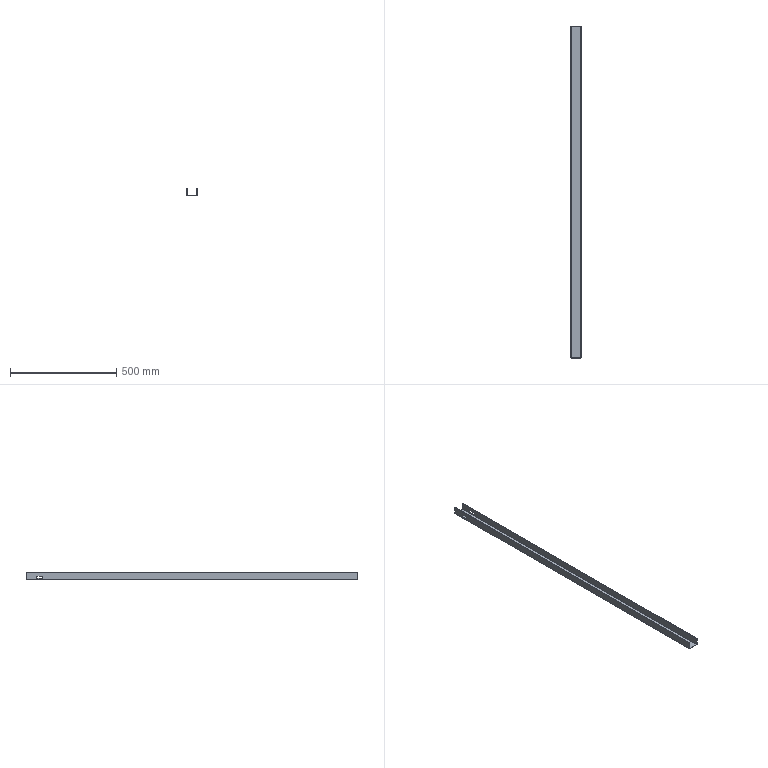Part | SolidWorks | features SplitBody 1 | 1 solid | 30 faces | box 50 x 1562 x 35 mm | volume 271759 mm3 | plane 26 | cylinder 4 | commonest cylinder face diameters 0.2 x2 3.2 x2
STEP:
#1=CARTESIAN_POINT('',(-25.,0.,-298.4));
#2=VERTEX_POINT('',#1);
#3=CARTESIAN_POINT('',(-23.5,0.,-298.4));
#4=VERTEX_POINT('',#3);
#5=CARTESIAN_POINT('',(-25.,0.,-298.4));
#6=DIRECTION('',(1.,0.,0.));
#7=VECTOR('',#6,1000.);
#8=LINE('',#5,#7);
#9=EDGE_CURVE('',#2,#4,#8,.T.);
#10=ORIENTED_EDGE('',*,*,#9,.F.);
#11=CARTESIAN_POINT('',(-23.4,0.,-300.));
#12=VERTEX_POINT('',#11);
#13=CARTESIAN_POINT('',(-23.4,0.,-298.4));
#14=DIRECTION('',(0.,-1.,0.));
#15=DIRECTION('',(0.,0.,1.));
#16=AXIS2_PLACEMENT_3D('',#13,#14,#15);
#17=CIRCLE('',#16,1.6);
#18=EDGE_CURVE('',#2,#12,#17,.T.);
#19=ORIENTED_EDGE('',*,*,#18,.T.);
#20=CARTESIAN_POINT('',(-23.4,0.,-298.5));
#21=VERTEX_POINT('',#20);
#22=CARTESIAN_POINT('',(-23.4,0.,-298.5));
#23=DIRECTION('',(0.,0.,-1.));
#24=VECTOR('',#23,1000.);
#25=LINE('',#22,#24);
#26=EDGE_CURVE('',#21,#12,#25,.T.);
#27=ORIENTED_EDGE('',*,*,#26,.F.);
#28=CARTESIAN_POINT('',(-23.4,0.,-298.4));
#29=DIRECTION('',(0.,-1.,0.));
#30=DIRECTION('',(1.,0.,0.));
#31=AXIS2_PLACEMENT_3D('',#28,#29,#30);
#32=CIRCLE('',#31,0.1);
#33=EDGE_CURVE('',#4,#21,#32,.T.);
#34=ORIENTED_EDGE('',*,*,#33,.F.);
#35=EDGE_LOOP('',(#10,#19,#27,#34));
#36=FACE_OUTER_BOUND('',#35,.T.);
#37=CARTESIAN_POINT('',(-25.,0.,-298.4));
#38=DIRECTION('',(0.,-1.,0.));
#39=DIRECTION('',(0.,0.,-1.));
#40=AXIS2_PLACEMENT_3D('',#37,#38,#39);
#41=PLANE('',#40);
#42=ADVANCED_FACE('',(#36),#41,.T.);
#43=CARTESIAN_POINT('',(-25.,0.,-265.));
#44=VERTEX_POINT('',#43);
#45=CARTESIAN_POINT('',(-25.,0.,-265.));
#46=DIRECTION('',(0.,0.,-1.));
#47=VECTOR('',#46,1000.);
#48=LINE('',#45,#47);
#49=EDGE_CURVE('',#44,#2,#48,.T.);
#50=ORIENTED_EDGE('',*,*,#49,.T.);
#51=ORIENTED_EDGE('',*,*,#9,.T.);
#52=CARTESIAN_POINT('',(-23.5,0.,-265.));
#53=VERTEX_POINT('',#52);
#54=CARTESIAN_POINT('',(-23.5,0.,-265.));
#55=DIRECTION('',(0.,0.,-1.));
#56=VECTOR('',#55,1000.);
#57=LINE('',#54,#56);
#58=EDGE_CURVE('',#53,#4,#57,.T.);
#59=ORIENTED_EDGE('',*,*,#58,.F.);
#60=CARTESIAN_POINT('',(-23.5,0.,-265.));
#61=DIRECTION('',(-1.,0.,0.));
#62=VECTOR('',#61,1000.);
#63=LINE('',#60,#62);
#64=EDGE_CURVE('',#53,#44,#63,.T.);
#65=ORIENTED_EDGE('',*,*,#64,.T.);
#66=EDGE_LOOP('',(#50,#51,#59,#65));
#67=FACE_OUTER_BOUND('',#66,.T.);
#68=CARTESIAN_POINT('',(-23.4,0.,-298.5));
#69=DIRECTION('',(0.,-1.,0.));
#70=DIRECTION('',(0.,0.,-1.));
#71=AXIS2_PLACEMENT_3D('',#68,#69,#70);
#72=PLANE('',#71);
#73=ADVANCED_FACE('',(#67),#72,.T.);
#74=CARTESIAN_POINT('',(23.4,0.,-300.));
#75=VERTEX_POINT('',#74);
#76=CARTESIAN_POINT('',(23.4,0.,-298.5));
#77=VERTEX_POINT('',#76);
#78=CARTESIAN_POINT('',(23.4,0.,-300.));
#79=DIRECTION('',(0.,0.,1.));
#80=VECTOR('',#79,1000.);
#81=LINE('',#78,#80);
#82=EDGE_CURVE('',#75,#77,#81,.T.);
#83=ORIENTED_EDGE('',*,*,#82,.F.);
#84=CARTESIAN_POINT('',(25.,0.,-298.4));
#85=VERTEX_POINT('',#84);
#86=CARTESIAN_POINT('',(23.4,0.,-298.4));
#87=DIRECTION('',(0.,-1.,0.));
#88=DIRECTION('',(0.,0.,1.));
#89=AXIS2_PLACEMENT_3D('',#86,#87,#88);
#90=CIRCLE('',#89,1.6);
#91=EDGE_CURVE('',#75,#85,#90,.T.);
#92=ORIENTED_EDGE('',*,*,#91,.T.);
#93=CARTESIAN_POINT('',(23.5,0.,-298.4));
#94=VERTEX_POINT('',#93);
#95=CARTESIAN_POINT('',(23.5,0.,-298.4));
#96=DIRECTION('',(1.,0.,0.));
#97=VECTOR('',#96,1000.);
#98=LINE('',#95,#97);
#99=EDGE_CURVE('',#94,#85,#98,.T.);
#100=ORIENTED_EDGE('',*,*,#99,.F.);
#101=CARTESIAN_POINT('',(23.4,0.,-298.4));
#102=DIRECTION('',(0.,-1.,0.));
#103=DIRECTION('',(1.,0.,0.));
#104=AXIS2_PLACEMENT_3D('',#101,#102,#103);
#105=CIRCLE('',#104,0.1);
#106=EDGE_CURVE('',#77,#94,#105,.T.);
#107=ORIENTED_EDGE('',*,*,#106,.F.);
#108=EDGE_LOOP('',(#83,#92,#100,#107));
#109=FACE_OUTER_BOUND('',#108,.T.);
#110=CARTESIAN_POINT('',(23.4,0.,-300.));
#111=DIRECTION('',(0.,-1.,0.));
#112=DIRECTION('',(0.,0.,-1.));
#113=AXIS2_PLACEMENT_3D('',#110,#111,#112);
#114=PLANE('',#113);
#115=ADVANCED_FACE('',(#109),#114,.T.);
#116=CARTESIAN_POINT('',(-25.,0.,-300.));
#117=DIRECTION('',(1.,0.,0.));
#118=VECTOR('',#117,1000.);
#119=LINE('',#116,#118);
#120=EDGE_CURVE('',#12,#75,#119,.T.);
#121=ORIENTED_EDGE('',*,*,#120,.T.);
#122=ORIENTED_EDGE('',*,*,#82,.T.);
#123=CARTESIAN_POINT('',(-25.,0.,-298.5));
#124=DIRECTION('',(1.,0.,0.));
#125=VECTOR('',#124,1000.);
#126=LINE('',#123,#125);
#127=EDGE_CURVE('',#21,#77,#126,.T.);
#128=ORIENTED_EDGE('',*,*,#127,.F.);
#129=ORIENTED_EDGE('',*,*,#26,.T.);
#130=EDGE_LOOP('',(#121,#122,#128,#129));
#131=FACE_OUTER_BOUND('',#130,.T.);
#132=CARTESIAN_POINT('',(23.5,0.,-298.4));
#133=DIRECTION('',(0.,-1.,0.));
#134=DIRECTION('',(0.,0.,-1.));
#135=AXIS2_PLACEMENT_3D('',#132,#133,#134);
#136=PLANE('',#135);
#137=ADVANCED_FACE('',(#131),#136,.T.);
#138=CARTESIAN_POINT('',(23.5,1486.25,-283.));
#139=VERTEX_POINT('',#138);
#140=CARTESIAN_POINT('',(23.5,1486.25,-293.));
#141=VERTEX_POINT('',#140);
#142=CARTESIAN_POINT('',(23.5,1486.25,-300.));
#143=DIRECTION('',(0.,0.,-1.));
#144=VECTOR('',#143,1000.);
#145=LINE('',#142,#144);
#146=EDGE_CURVE('',#139,#141,#145,.T.);
#147=ORIENTED_EDGE('',*,*,#146,.T.);
#148=CARTESIAN_POINT('',(23.5,1511.25,-293.));
#149=VERTEX_POINT('',#148);
#150=CARTESIAN_POINT('',(23.5,1623.533,-293.));
#151=DIRECTION('',(0.,1.,0.));
#152=VECTOR('',#151,1000.);
#153=LINE('',#150,#152);
#154=EDGE_CURVE('',#141,#149,#153,.T.);
#155=ORIENTED_EDGE('',*,*,#154,.T.);
#156=CARTESIAN_POINT('',(23.5,1511.25,-283.));
#157=VERTEX_POINT('',#156);
#158=CARTESIAN_POINT('',(23.5,1511.25,-300.));
#159=DIRECTION('',(0.,0.,1.));
#160=VECTOR('',#159,1000.);
#161=LINE('',#158,#160);
#162=EDGE_CURVE('',#149,#157,#161,.T.);
#163=ORIENTED_EDGE('',*,*,#162,.T.);
#164=CARTESIAN_POINT('',(23.5,1623.533,-283.));
#165=DIRECTION('',(0.,-1.,0.));
#166=VECTOR('',#165,1000.);
#167=LINE('',#164,#166);
#168=EDGE_CURVE('',#157,#139,#167,.T.);
#169=ORIENTED_EDGE('',*,*,#168,.T.);
#170=EDGE_LOOP('',(#147,#155,#163,#169));
#171=FACE_BOUND('',#170,.T.);
#172=CARTESIAN_POINT('',(23.5,1562.5,-298.4));
#173=VERTEX_POINT('',#172);
#174=CARTESIAN_POINT('',(23.5,1562.5,-265.));
#175=VERTEX_POINT('',#174);
#176=CARTESIAN_POINT('',(23.5,1562.5,-300.));
#177=DIRECTION('',(0.,0.,1.));
#178=VECTOR('',#177,1000.);
#179=LINE('',#176,#178);
#180=EDGE_CURVE('',#173,#175,#179,.T.);
#181=ORIENTED_EDGE('',*,*,#180,.F.);
#182=CARTESIAN_POINT('',(23.5,1623.533,-298.4));
#183=DIRECTION('',(0.,-1.,0.));
#184=VECTOR('',#183,1000.);
#185=LINE('',#182,#184);
#186=EDGE_CURVE('',#173,#94,#185,.T.);
#187=ORIENTED_EDGE('',*,*,#186,.T.);
#188=CARTESIAN_POINT('',(23.5,0.,-265.));
#189=VERTEX_POINT('',#188);
#190=CARTESIAN_POINT('',(23.5,0.,-300.));
#191=DIRECTION('',(0.,0.,1.));
#192=VECTOR('',#191,1000.);
#193=LINE('',#190,#192);
#194=EDGE_CURVE('',#94,#189,#193,.T.);
#195=ORIENTED_EDGE('',*,*,#194,.T.);
#196=CARTESIAN_POINT('',(23.5,1623.533,-265.));
#197=DIRECTION('',(0.,-1.,0.));
#198=VECTOR('',#197,1000.);
#199=LINE('',#196,#198);
#200=EDGE_CURVE('',#175,#189,#199,.T.);
#201=ORIENTED_EDGE('',*,*,#200,.F.);
#202=EDGE_LOOP('',(#181,#187,#195,#201));
#203=FACE_OUTER_BOUND('',#202,.T.);
#204=CARTESIAN_POINT('',(23.5,1623.533,-300.));
#205=DIRECTION('',(1.,0.,0.));
#206=DIRECTION('',(0.,0.,-1.));
#207=AXIS2_PLACEMENT_3D('',#204,#205,#206);
#208=PLANE('',#207);
#209=ADVANCED_FACE('',(#171,#203),#208,.F.);
#210=CARTESIAN_POINT('',(25.,1562.5,-265.));
#211=VERTEX_POINT('',#210);
#212=CARTESIAN_POINT('',(25.,0.,-265.));
#213=VERTEX_POINT('',#212);
#214=CARTESIAN_POINT('',(25.,1623.533,-265.));
#215=DIRECTION('',(0.,-1.,0.));
#216=VECTOR('',#215,1000.);
#217=LINE('',#214,#216);
#218=EDGE_CURVE('',#211,#213,#217,.T.);
#219=ORIENTED_EDGE('',*,*,#218,.F.);
#220=CARTESIAN_POINT('',(25.,1562.5,-265.));
#221=DIRECTION('',(-1.,0.,0.));
#222=VECTOR('',#221,1000.);
#223=LINE('',#220,#222);
#224=EDGE_CURVE('',#211,#175,#223,.T.);
#225=ORIENTED_EDGE('',*,*,#224,.T.);
#226=ORIENTED_EDGE('',*,*,#200,.T.);
#227=CARTESIAN_POINT('',(25.,0.,-265.));
#228=DIRECTION('',(-1.,0.,0.));
#229=VECTOR('',#228,1000.);
#230=LINE('',#227,#229);
#231=EDGE_CURVE('',#213,#189,#230,.T.);
#232=ORIENTED_EDGE('',*,*,#231,.F.);
#233=EDGE_LOOP('',(#219,#225,#226,#232));
#234=FACE_OUTER_BOUND('',#233,.T.);
#235=CARTESIAN_POINT('',(25.,1623.533,-265.));
#236=DIRECTION('',(0.,0.,1.));
#237=DIRECTION('',(1.,0.,0.));
#238=AXIS2_PLACEMENT_3D('',#235,#236,#237);
#239=PLANE('',#238);
#240=ADVANCED_FACE('',(#234),#239,.T.);
#241=CARTESIAN_POINT('',(25.,1486.25,-293.));
#242=VERTEX_POINT('',#241);
#243=CARTESIAN_POINT('',(25.,1511.25,-293.));
#244=VERTEX_POINT('',#243);
#245=CARTESIAN_POINT('',(25.,1511.25,-293.));
#246=DIRECTION('',(0.,1.,0.));
#247=VECTOR('',#246,1000.);
#248=LINE('',#245,#247);
#249=EDGE_CURVE('',#242,#244,#248,.T.);
#250=ORIENTED_EDGE('',*,*,#249,.F.);
#251=CARTESIAN_POINT('',(25.,1486.25,-283.));
#252=VERTEX_POINT('',#251);
#253=CARTESIAN_POINT('',(25.,1486.25,-293.));
#254=DIRECTION('',(0.,0.,-1.));
#255=VECTOR('',#254,1000.);
#256=LINE('',#253,#255);
#257=EDGE_CURVE('',#252,#242,#256,.T.);
#258=ORIENTED_EDGE('',*,*,#257,.F.);
#259=CARTESIAN_POINT('',(25.,1511.25,-283.));
#260=VERTEX_POINT('',#259);
#261=CARTESIAN_POINT('',(25.,1511.25,-283.));
#262=DIRECTION('',(0.,-1.,0.));
#263=VECTOR('',#262,1000.);
#264=LINE('',#261,#263);
#265=EDGE_CURVE('',#260,#252,#264,.T.);
#266=ORIENTED_EDGE('',*,*,#265,.F.);
#267=CARTESIAN_POINT('',(25.,1511.25,-293.));
#268=DIRECTION('',(0.,0.,1.));
#269=VECTOR('',#268,1000.);
#270=LINE('',#267,#269);
#271=EDGE_CURVE('',#244,#260,#270,.T.);
#272=ORIENTED_EDGE('',*,*,#271,.F.);
#273=EDGE_LOOP('',(#250,#258,#266,#272));
#274=FACE_BOUND('',#273,.T.);
#275=CARTESIAN_POINT('',(25.,1562.5,-298.4));
#276=VERTEX_POINT('',#275);
#277=CARTESIAN_POINT('',(25.,1623.533,-298.4));
#278=DIRECTION('',(0.,-1.,0.));
#279=VECTOR('',#278,1000.);
#280=LINE('',#277,#279);
#281=EDGE_CURVE('',#276,#85,#280,.T.);
#282=ORIENTED_EDGE('',*,*,#281,.F.);
#283=CARTESIAN_POINT('',(25.,1562.5,-300.));
#284=DIRECTION('',(0.,0.,1.));
#285=VECTOR('',#284,1000.);
#286=LINE('',#283,#285);
#287=EDGE_CURVE('',#276,#211,#286,.T.);
#288=ORIENTED_EDGE('',*,*,#287,.T.);
#289=ORIENTED_EDGE('',*,*,#218,.T.);
#290=CARTESIAN_POINT('',(25.,0.,-300.));
#291=DIRECTION('',(0.,0.,1.));
#292=VECTOR('',#291,1000.);
#293=LINE('',#290,#292);
#294=EDGE_CURVE('',#85,#213,#293,.T.);
#295=ORIENTED_EDGE('',*,*,#294,.F.);
#296=EDGE_LOOP('',(#282,#288,#289,#295));
#297=FACE_OUTER_BOUND('',#296,.T.);
#298=CARTESIAN_POINT('',(25.,1623.533,-300.));
#299=DIRECTION('',(1.,0.,0.));
#300=DIRECTION('',(0.,0.,-1.));
#301=AXIS2_PLACEMENT_3D('',#298,#299,#300);
#302=PLANE('',#301);
#303=ADVANCED_FACE('',(#274,#297),#302,.T.);
#304=CARTESIAN_POINT('',(23.4,1562.5,-300.));
#305=VERTEX_POINT('',#304);
#306=CARTESIAN_POINT('',(23.4,1623.533,-300.));
#307=DIRECTION('',(0.,-1.,0.));
#308=VECTOR('',#307,1000.);
#309=LINE('',#306,#308);
#310=EDGE_CURVE('',#305,#75,#309,.T.);
#311=ORIENTED_EDGE('',*,*,#310,.F.);
#312=CARTESIAN_POINT('',(23.4,1562.5,-298.4));
#313=DIRECTION('',(0.,1.,0.));
#314=DIRECTION('',(0.,0.,-1.));
#315=AXIS2_PLACEMENT_3D('',#312,#313,#314);
#316=CIRCLE('',#315,1.6);
#317=EDGE_CURVE('',#276,#305,#316,.T.);
#318=ORIENTED_EDGE('',*,*,#317,.F.);
#319=ORIENTED_EDGE('',*,*,#281,.T.);
#320=ORIENTED_EDGE('',*,*,#91,.F.);
#321=EDGE_LOOP('',(#311,#318,#319,#320));
#322=FACE_OUTER_BOUND('',#321,.T.);
#323=CARTESIAN_POINT('',(23.4,1623.533,-298.4));
#324=DIRECTION('',(0.,-1.,0.));
#325=DIRECTION('',(0.,0.,-1.));
#326=AXIS2_PLACEMENT_3D('',#323,#324,#325);
#327=CYLINDRICAL_SURFACE('',#326,1.6);
#328=ADVANCED_FACE('',(#322),#327,.T.);
#329=CARTESIAN_POINT('',(-23.4,1562.5,-300.));
#330=VERTEX_POINT('',#329);
#331=CARTESIAN_POINT('',(-23.4,1623.533,-300.));
#332=DIRECTION('',(0.,-1.,0.));
#333=VECTOR('',#332,1000.);
#334=LINE('',#331,#333);
#335=EDGE_CURVE('',#330,#12,#334,.T.);
#336=ORIENTED_EDGE('',*,*,#335,.F.);
#337=CARTESIAN_POINT('',(-25.,1562.5,-300.));
#338=DIRECTION('',(1.,0.,0.));
#339=VECTOR('',#338,1000.);
#340=LINE('',#337,#339);
#341=EDGE_CURVE('',#330,#305,#340,.T.);
#342=ORIENTED_EDGE('',*,*,#341,.T.);
#343=ORIENTED_EDGE('',*,*,#310,.T.);
#344=ORIENTED_EDGE('',*,*,#120,.F.);
#345=EDGE_LOOP('',(#336,#342,#343,#344));
#346=FACE_OUTER_BOUND('',#345,.T.);
#347=CARTESIAN_POINT('',(-25.,1623.533,-300.));
#348=DIRECTION('',(0.,0.,-1.));
#349=DIRECTION('',(-1.,0.,0.));
#350=AXIS2_PLACEMENT_3D('',#347,#348,#349);
#351=PLANE('',#350);
#352=ADVANCED_FACE('',(#346),#351,.T.);
#353=CARTESIAN_POINT('',(-25.,1562.5,-298.4));
#354=VERTEX_POINT('',#353);
#355=CARTESIAN_POINT('',(-25.,1623.533,-298.4));
#356=DIRECTION('',(0.,-1.,0.));
#357=VECTOR('',#356,1000.);
#358=LINE('',#355,#357);
#359=EDGE_CURVE('',#354,#2,#358,.T.);
#360=ORIENTED_EDGE('',*,*,#359,.F.);
#361=CARTESIAN_POINT('',(-23.4,1562.5,-298.4));
#362=DIRECTION('',(0.,1.,0.));
#363=DIRECTION('',(0.,0.,-1.));
#364=AXIS2_PLACEMENT_3D('',#361,#362,#363);
#365=CIRCLE('',#364,1.6);
#366=EDGE_CURVE('',#330,#354,#365,.T.);
#367=ORIENTED_EDGE('',*,*,#366,.F.);
#368=ORIENTED_EDGE('',*,*,#335,.T.);
#369=ORIENTED_EDGE('',*,*,#18,.F.);
#370=EDGE_LOOP('',(#360,#367,#368,#369));
#371=FACE_OUTER_BOUND('',#370,.T.);
#372=CARTESIAN_POINT('',(-23.4,1623.533,-298.4));
#373=DIRECTION('',(0.,-1.,0.));
#374=DIRECTION('',(0.,0.,-1.));
#375=AXIS2_PLACEMENT_3D('',#372,#373,#374);
#376=CYLINDRICAL_SURFACE('',#375,1.6);
#377=ADVANCED_FACE('',(#371),#376,.T.);
#378=CARTESIAN_POINT('',(-25.,1511.25,-293.));
#379=VERTEX_POINT('',#378);
#380=CARTESIAN_POINT('',(-25.,1486.25,-293.));
#381=VERTEX_POINT('',#380);
#382=CARTESIAN_POINT('',(-25.,1623.533,-293.));
#383=DIRECTION('',(0.,-1.,0.));
#384=VECTOR('',#383,1000.);
#385=LINE('',#382,#384);
#386=EDGE_CURVE('',#379,#381,#385,.T.);
#387=ORIENTED_EDGE('',*,*,#386,.F.);
#388=CARTESIAN_POINT('',(-25.,1511.25,-283.));
#389=VERTEX_POINT('',#388);
#390=CARTESIAN_POINT('',(-25.,1511.25,-265.));
#391=DIRECTION('',(0.,0.,-1.));
#392=VECTOR('',#391,1000.);
#393=LINE('',#390,#392);
#394=EDGE_CURVE('',#389,#379,#393,.T.);
#395=ORIENTED_EDGE('',*,*,#394,.F.);
#396=CARTESIAN_POINT('',(-25.,1486.25,-283.));
#397=VERTEX_POINT('',#396);
#398=CARTESIAN_POINT('',(-25.,1623.533,-283.));
#399=DIRECTION('',(0.,1.,0.));
#400=VECTOR('',#399,1000.);
#401=LINE('',#398,#400);
#402=EDGE_CURVE('',#397,#389,#401,.T.);
#403=ORIENTED_EDGE('',*,*,#402,.F.);
#404=CARTESIAN_POINT('',(-25.,1486.25,-265.));
#405=DIRECTION('',(0.,0.,1.));
#406=VECTOR('',#405,1000.);
#407=LINE('',#404,#406);
#408=EDGE_CURVE('',#381,#397,#407,.T.);
#409=ORIENTED_EDGE('',*,*,#408,.F.);
#410=EDGE_LOOP('',(#387,#395,#403,#409));
#411=FACE_BOUND('',#410,.T.);
#412=CARTESIAN_POINT('',(-25.,1562.5,-265.));
#413=VERTEX_POINT('',#412);
#414=CARTESIAN_POINT('',(-25.,1623.533,-265.));
#415=DIRECTION('',(0.,-1.,0.));
#416=VECTOR('',#415,1000.);
#417=LINE('',#414,#416);
#418=EDGE_CURVE('',#413,#44,#417,.T.);
#419=ORIENTED_EDGE('',*,*,#418,.F.);
#420=CARTESIAN_POINT('',(-25.,1562.5,-265.));
#421=DIRECTION('',(0.,0.,-1.));
#422=VECTOR('',#421,1000.);
#423=LINE('',#420,#422);
#424=EDGE_CURVE('',#413,#354,#423,.T.);
#425=ORIENTED_EDGE('',*,*,#424,.T.);
#426=ORIENTED_EDGE('',*,*,#359,.T.);
#427=ORIENTED_EDGE('',*,*,#49,.F.);
#428=EDGE_LOOP('',(#419,#425,#426,#427));
#429=FACE_OUTER_BOUND('',#428,.T.);
#430=CARTESIAN_POINT('',(-25.,1623.533,-265.));
#431=DIRECTION('',(-1.,0.,0.));
#432=DIRECTION('',(0.,0.,1.));
#433=AXIS2_PLACEMENT_3D('',#430,#431,#432);
#434=PLANE('',#433);
#435=ADVANCED_FACE('',(#411,#429),#434,.T.);
#436=CARTESIAN_POINT('',(-23.5,1562.5,-265.));
#437=VERTEX_POINT('',#436);
#438=CARTESIAN_POINT('',(-23.5,1623.533,-265.));
#439=DIRECTION('',(0.,-1.,0.));
#440=VECTOR('',#439,1000.);
#441=LINE('',#438,#440);
#442=EDGE_CURVE('',#437,#53,#441,.T.);
#443=ORIENTED_EDGE('',*,*,#442,.F.);
#444=CARTESIAN_POINT('',(-23.5,1562.5,-265.));
#445=DIRECTION('',(-1.,0.,0.));
#446=VECTOR('',#445,1000.);
#447=LINE('',#444,#446);
#448=EDGE_CURVE('',#437,#413,#447,.T.);
#449=ORIENTED_EDGE('',*,*,#448,.T.);
#450=ORIENTED_EDGE('',*,*,#418,.T.);
#451=ORIENTED_EDGE('',*,*,#64,.F.);
#452=EDGE_LOOP('',(#443,#449,#450,#451));
#453=FACE_OUTER_BOUND('',#452,.T.);
#454=CARTESIAN_POINT('',(-23.5,1623.533,-265.));
#455=DIRECTION('',(0.,0.,1.));
#456=DIRECTION('',(1.,0.,0.));
#457=AXIS2_PLACEMENT_3D('',#454,#455,#456);
#458=PLANE('',#457);
#459=ADVANCED_FACE('',(#453),#458,.T.);
#460=CARTESIAN_POINT('',(-23.5,1511.25,-283.));
#461=VERTEX_POINT('',#460);
#462=CARTESIAN_POINT('',(-23.5,1511.25,-293.));
#463=VERTEX_POINT('',#462);
#464=CARTESIAN_POINT('',(-23.5,1511.25,-265.));
#465=DIRECTION('',(0.,0.,-1.));
#466=VECTOR('',#465,1000.);
#467=LINE('',#464,#466);
#468=EDGE_CURVE('',#461,#463,#467,.T.);
#469=ORIENTED_EDGE('',*,*,#468,.T.);
#470=CARTESIAN_POINT('',(-23.5,1486.25,-293.));
#471=VERTEX_POINT('',#470);
#472=CARTESIAN_POINT('',(-23.5,1623.533,-293.));
#473=DIRECTION('',(0.,-1.,0.));
#474=VECTOR('',#473,1000.);
#475=LINE('',#472,#474);
#476=EDGE_CURVE('',#463,#471,#475,.T.);
#477=ORIENTED_EDGE('',*,*,#476,.T.);
#478=CARTESIAN_POINT('',(-23.5,1486.25,-283.));
#479=VERTEX_POINT('',#478);
#480=CARTESIAN_POINT('',(-23.5,1486.25,-265.));
#481=DIRECTION('',(0.,0.,1.));
#482=VECTOR('',#481,1000.);
#483=LINE('',#480,#482);
#484=EDGE_CURVE('',#471,#479,#483,.T.);
#485=ORIENTED_EDGE('',*,*,#484,.T.);
#486=CARTESIAN_POINT('',(-23.5,1623.533,-283.));
#487=DIRECTION('',(0.,1.,0.));
#488=VECTOR('',#487,1000.);
#489=LINE('',#486,#488);
#490=EDGE_CURVE('',#479,#461,#489,.T.);
#491=ORIENTED_EDGE('',*,*,#490,.T.);
#492=EDGE_LOOP('',(#469,#477,#485,#491));
#493=FACE_BOUND('',#492,.T.);
#494=CARTESIAN_POINT('',(-23.5,1562.5,-298.4));
#495=VERTEX_POINT('',#494);
#496=CARTESIAN_POINT('',(-23.5,1562.5,-265.));
#497=DIRECTION('',(0.,0.,-1.));
#498=VECTOR('',#497,1000.);
#499=LINE('',#496,#498);
#500=EDGE_CURVE('',#437,#495,#499,.T.);
#501=ORIENTED_EDGE('',*,*,#500,.F.);
#502=ORIENTED_EDGE('',*,*,#442,.T.);
#503=ORIENTED_EDGE('',*,*,#58,.T.);
#504=CARTESIAN_POINT('',(-23.5,1623.533,-298.4));
#505=DIRECTION('',(0.,-1.,0.));
#506=VECTOR('',#505,1000.);
#507=LINE('',#504,#506);
#508=EDGE_CURVE('',#495,#4,#507,.T.);
#509=ORIENTED_EDGE('',*,*,#508,.F.);
#510=EDGE_LOOP('',(#501,#502,#503,#509));
#511=FACE_OUTER_BOUND('',#510,.T.);
#512=CARTESIAN_POINT('',(-23.5,1623.533,-265.));
#513=DIRECTION('',(-1.,0.,0.));
#514=DIRECTION('',(0.,0.,1.));
#515=AXIS2_PLACEMENT_3D('',#512,#513,#514);
#516=PLANE('',#515);
#517=ADVANCED_FACE('',(#493,#511),#516,.F.);
#518=CARTESIAN_POINT('',(-23.4,1562.5,-298.5));
#519=VERTEX_POINT('',#518);
#520=CARTESIAN_POINT('',(-23.4,1562.5,-298.4));
#521=DIRECTION('',(0.,-1.,0.));
#522=DIRECTION('',(0.,0.,1.));
#523=AXIS2_PLACEMENT_3D('',#520,#521,#522);
#524=CIRCLE('',#523,0.1);
#525=EDGE_CURVE('',#495,#519,#524,.T.);
#526=ORIENTED_EDGE('',*,*,#525,.F.);
#527=ORIENTED_EDGE('',*,*,#508,.T.);
#528=ORIENTED_EDGE('',*,*,#33,.T.);
#529=CARTESIAN_POINT('',(-23.4,1623.533,-298.5));
#530=DIRECTION('',(0.,-1.,0.));
#531=VECTOR('',#530,1000.);
#532=LINE('',#529,#531);
#533=EDGE_CURVE('',#519,#21,#532,.T.);
#534=ORIENTED_EDGE('',*,*,#533,.F.);
#535=EDGE_LOOP('',(#526,#527,#528,#534));
#536=FACE_OUTER_BOUND('',#535,.T.);
#537=CARTESIAN_POINT('',(-23.4,1623.533,-298.4));
#538=DIRECTION('',(0.,-1.,0.));
#539=DIRECTION('',(0.,0.,-1.));
#540=AXIS2_PLACEMENT_3D('',#537,#538,#539);
#541=CYLINDRICAL_SURFACE('',#540,0.1);
#542=ADVANCED_FACE('',(#536),#541,.F.);
#543=CARTESIAN_POINT('',(23.4,1562.5,-298.5));
#544=VERTEX_POINT('',#543);
#545=CARTESIAN_POINT('',(-25.,1562.5,-298.5));
#546=DIRECTION('',(1.,0.,0.));
#547=VECTOR('',#546,1000.);
#548=LINE('',#545,#547);
#549=EDGE_CURVE('',#519,#544,#548,.T.);
#550=ORIENTED_EDGE('',*,*,#549,.F.);
#551=ORIENTED_EDGE('',*,*,#533,.T.);
#552=ORIENTED_EDGE('',*,*,#127,.T.);
#553=CARTESIAN_POINT('',(23.4,1623.533,-298.5));
#554=DIRECTION('',(0.,-1.,0.));
#555=VECTOR('',#554,1000.);
#556=LINE('',#553,#555);
#557=EDGE_CURVE('',#544,#77,#556,.T.);
#558=ORIENTED_EDGE('',*,*,#557,.F.);
#559=EDGE_LOOP('',(#550,#551,#552,#558));
#560=FACE_OUTER_BOUND('',#559,.T.);
#561=CARTESIAN_POINT('',(-25.,1623.533,-298.5));
#562=DIRECTION('',(0.,0.,-1.));
#563=DIRECTION('',(-1.,0.,0.));
#564=AXIS2_PLACEMENT_3D('',#561,#562,#563);
#565=PLANE('',#564);
#566=ADVANCED_FACE('',(#560),#565,.F.);
#567=CARTESIAN_POINT('',(23.4,1562.5,-298.4));
#568=DIRECTION('',(0.,-1.,0.));
#569=DIRECTION('',(0.,0.,1.));
#570=AXIS2_PLACEMENT_3D('',#567,#568,#569);
#571=CIRCLE('',#570,0.1);
#572=EDGE_CURVE('',#544,#173,#571,.T.);
#573=ORIENTED_EDGE('',*,*,#572,.F.);
#574=ORIENTED_EDGE('',*,*,#557,.T.);
#575=ORIENTED_EDGE('',*,*,#106,.T.);
#576=ORIENTED_EDGE('',*,*,#186,.F.);
#577=EDGE_LOOP('',(#573,#574,#575,#576));
#578=FACE_OUTER_BOUND('',#577,.T.);
#579=CARTESIAN_POINT('',(23.4,1623.533,-298.4));
#580=DIRECTION('',(0.,-1.,0.));
#581=DIRECTION('',(0.,0.,-1.));
#582=AXIS2_PLACEMENT_3D('',#579,#580,#581);
#583=CYLINDRICAL_SURFACE('',#582,0.1);
#584=ADVANCED_FACE('',(#578),#583,.F.);
#585=ORIENTED_EDGE('',*,*,#194,.F.);
#586=ORIENTED_EDGE('',*,*,#99,.T.);
#587=ORIENTED_EDGE('',*,*,#294,.T.);
#588=ORIENTED_EDGE('',*,*,#231,.T.);
#589=EDGE_LOOP('',(#585,#586,#587,#588));
#590=FACE_OUTER_BOUND('',#589,.T.);
#591=CARTESIAN_POINT('',(23.4,0.,-298.4));
#592=DIRECTION('',(0.,1.,0.));
#593=DIRECTION('',(1.,0.,0.));
#594=AXIS2_PLACEMENT_3D('',#591,#592,#593);
#595=PLANE('',#594);
#596=ADVANCED_FACE('',(#590),#595,.F.);
#597=ORIENTED_EDGE('',*,*,#549,.T.);
#598=CARTESIAN_POINT('',(23.4,1562.5,-298.5));
#599=DIRECTION('',(0.,0.,-1.));
#600=VECTOR('',#599,1000.);
#601=LINE('',#598,#600);
#602=EDGE_CURVE('',#544,#305,#601,.T.);
#603=ORIENTED_EDGE('',*,*,#602,.T.);
#604=ORIENTED_EDGE('',*,*,#341,.F.);
#605=CARTESIAN_POINT('',(-23.4,1562.5,-298.5));
#606=DIRECTION('',(0.,0.,-1.));
#607=VECTOR('',#606,1000.);
#608=LINE('',#605,#607);
#609=EDGE_CURVE('',#519,#330,#608,.T.);
#610=ORIENTED_EDGE('',*,*,#609,.F.);
#611=EDGE_LOOP('',(#597,#603,#604,#610));
#612=FACE_OUTER_BOUND('',#611,.T.);
#613=CARTESIAN_POINT('',(-25.,1562.5,-298.5));
#614=DIRECTION('',(0.,1.,0.));
#615=DIRECTION('',(1.,0.,0.));
#616=AXIS2_PLACEMENT_3D('',#613,#614,#615);
#617=PLANE('',#616);
#618=ADVANCED_FACE('',(#612),#617,.T.);
#619=ORIENTED_EDGE('',*,*,#500,.T.);
#620=CARTESIAN_POINT('',(-23.5,1562.5,-298.4));
#621=DIRECTION('',(-1.,0.,0.));
#622=VECTOR('',#621,1000.);
#623=LINE('',#620,#622);
#624=EDGE_CURVE('',#495,#354,#623,.T.);
#625=ORIENTED_EDGE('',*,*,#624,.T.);
#626=ORIENTED_EDGE('',*,*,#424,.F.);
#627=ORIENTED_EDGE('',*,*,#448,.F.);
#628=EDGE_LOOP('',(#619,#625,#626,#627));
#629=FACE_OUTER_BOUND('',#628,.T.);
#630=CARTESIAN_POINT('',(-23.5,1562.5,-265.));
#631=DIRECTION('',(0.,1.,0.));
#632=DIRECTION('',(0.,0.,-1.));
#633=AXIS2_PLACEMENT_3D('',#630,#631,#632);
#634=PLANE('',#633);
#635=ADVANCED_FACE('',(#629),#634,.T.);
#636=ORIENTED_EDGE('',*,*,#366,.T.);
#637=ORIENTED_EDGE('',*,*,#624,.F.);
#638=ORIENTED_EDGE('',*,*,#525,.T.);
#639=ORIENTED_EDGE('',*,*,#609,.T.);
#640=EDGE_LOOP('',(#636,#637,#638,#639));
#641=FACE_OUTER_BOUND('',#640,.T.);
#642=CARTESIAN_POINT('',(-23.4,1562.5,-298.4));
#643=DIRECTION('',(0.,-1.,0.));
#644=DIRECTION('',(0.,0.,-1.));
#645=AXIS2_PLACEMENT_3D('',#642,#643,#644);
#646=PLANE('',#645);
#647=ADVANCED_FACE('',(#641),#646,.F.);
#648=ORIENTED_EDGE('',*,*,#224,.F.);
#649=ORIENTED_EDGE('',*,*,#287,.F.);
#650=CARTESIAN_POINT('',(25.,1562.5,-298.4));
#651=DIRECTION('',(-1.,0.,0.));
#652=VECTOR('',#651,1000.);
#653=LINE('',#650,#652);
#654=EDGE_CURVE('',#276,#173,#653,.T.);
#655=ORIENTED_EDGE('',*,*,#654,.T.);
#656=ORIENTED_EDGE('',*,*,#180,.T.);
#657=EDGE_LOOP('',(#648,#649,#655,#656));
#658=FACE_OUTER_BOUND('',#657,.T.);
#659=CARTESIAN_POINT('',(25.,1562.5,-300.));
#660=DIRECTION('',(0.,1.,0.));
#661=DIRECTION('',(0.,0.,1.));
#662=AXIS2_PLACEMENT_3D('',#659,#660,#661);
#663=PLANE('',#662);
#664=ADVANCED_FACE('',(#658),#663,.T.);
#665=ORIENTED_EDGE('',*,*,#317,.T.);
#666=ORIENTED_EDGE('',*,*,#602,.F.);
#667=ORIENTED_EDGE('',*,*,#572,.T.);
#668=ORIENTED_EDGE('',*,*,#654,.F.);
#669=EDGE_LOOP('',(#665,#666,#667,#668));
#670=FACE_OUTER_BOUND('',#669,.T.);
#671=CARTESIAN_POINT('',(23.4,1562.5,-298.4));
#672=DIRECTION('',(0.,-1.,0.));
#673=DIRECTION('',(0.,0.,-1.));
#674=AXIS2_PLACEMENT_3D('',#671,#672,#673);
#675=PLANE('',#674);
#676=ADVANCED_FACE('',(#670),#675,.F.);
#677=ORIENTED_EDGE('',*,*,#394,.T.);
#678=CARTESIAN_POINT('',(-550.,1511.25,-293.));
#679=DIRECTION('',(1.,0.,0.));
#680=VECTOR('',#679,1000.);
#681=LINE('',#678,#680);
#682=EDGE_CURVE('',#379,#463,#681,.T.);
#683=ORIENTED_EDGE('',*,*,#682,.T.);
#684=ORIENTED_EDGE('',*,*,#468,.F.);
#685=CARTESIAN_POINT('',(-550.,1511.25,-283.));
#686=DIRECTION('',(1.,0.,0.));
#687=VECTOR('',#686,1000.);
#688=LINE('',#685,#687);
#689=EDGE_CURVE('',#389,#461,#688,.T.);
#690=ORIENTED_EDGE('',*,*,#689,.F.);
#691=EDGE_LOOP('',(#677,#683,#684,#690));
#692=FACE_OUTER_BOUND('',#691,.T.);
#693=CARTESIAN_POINT('',(-550.,1511.25,-293.));
#694=DIRECTION('',(0.,1.,0.));
#695=DIRECTION('',(0.,0.,1.));
#696=AXIS2_PLACEMENT_3D('',#693,#694,#695);
#697=PLANE('',#696);
#698=ADVANCED_FACE('',(#692),#697,.F.);
#699=ORIENTED_EDGE('',*,*,#402,.T.);
#700=ORIENTED_EDGE('',*,*,#689,.T.);
#701=ORIENTED_EDGE('',*,*,#490,.F.);
#702=CARTESIAN_POINT('',(-550.,1486.25,-283.));
#703=DIRECTION('',(1.,0.,0.));
#704=VECTOR('',#703,1000.);
#705=LINE('',#702,#704);
#706=EDGE_CURVE('',#397,#479,#705,.T.);
#707=ORIENTED_EDGE('',*,*,#706,.F.);
#708=EDGE_LOOP('',(#699,#700,#701,#707));
#709=FACE_OUTER_BOUND('',#708,.T.);
#710=CARTESIAN_POINT('',(-550.,1511.25,-283.));
#711=DIRECTION('',(0.,0.,1.));
#712=DIRECTION('',(1.,0.,0.));
#713=AXIS2_PLACEMENT_3D('',#710,#711,#712);
#714=PLANE('',#713);
#715=ADVANCED_FACE('',(#709),#714,.F.);
#716=ORIENTED_EDGE('',*,*,#408,.T.);
#717=ORIENTED_EDGE('',*,*,#706,.T.);
#718=ORIENTED_EDGE('',*,*,#484,.F.);
#719=CARTESIAN_POINT('',(-550.,1486.25,-293.));
#720=DIRECTION('',(1.,0.,0.));
#721=VECTOR('',#720,1000.);
#722=LINE('',#719,#721);
#723=EDGE_CURVE('',#381,#471,#722,.T.);
#724=ORIENTED_EDGE('',*,*,#723,.F.);
#725=EDGE_LOOP('',(#716,#717,#718,#724));
#726=FACE_OUTER_BOUND('',#725,.T.);
#727=CARTESIAN_POINT('',(-550.,1486.25,-293.));
#728=DIRECTION('',(0.,-1.,0.));
#729=DIRECTION('',(0.,0.,-1.));
#730=AXIS2_PLACEMENT_3D('',#727,#728,#729);
#731=PLANE('',#730);
#732=ADVANCED_FACE('',(#726),#731,.F.);
#733=ORIENTED_EDGE('',*,*,#386,.T.);
#734=ORIENTED_EDGE('',*,*,#723,.T.);
#735=ORIENTED_EDGE('',*,*,#476,.F.);
#736=ORIENTED_EDGE('',*,*,#682,.F.);
#737=EDGE_LOOP('',(#733,#734,#735,#736));
#738=FACE_OUTER_BOUND('',#737,.T.);
#739=CARTESIAN_POINT('',(-550.,1511.25,-293.));
#740=DIRECTION('',(0.,0.,-1.));
#741=DIRECTION('',(-1.,0.,0.));
#742=AXIS2_PLACEMENT_3D('',#739,#740,#741);
#743=PLANE('',#742);
#744=ADVANCED_FACE('',(#738),#743,.F.);
#745=CARTESIAN_POINT('',(-550.,1486.25,-293.));
#746=DIRECTION('',(1.,0.,0.));
#747=VECTOR('',#746,1000.);
#748=LINE('',#745,#747);
#749=EDGE_CURVE('',#141,#242,#748,.T.);
#750=ORIENTED_EDGE('',*,*,#749,.T.);
#751=ORIENTED_EDGE('',*,*,#249,.T.);
#752=CARTESIAN_POINT('',(-550.,1511.25,-293.));
#753=DIRECTION('',(1.,0.,0.));
#754=VECTOR('',#753,1000.);
#755=LINE('',#752,#754);
#756=EDGE_CURVE('',#149,#244,#755,.T.);
#757=ORIENTED_EDGE('',*,*,#756,.F.);
#758=ORIENTED_EDGE('',*,*,#154,.F.);
#759=EDGE_LOOP('',(#750,#751,#757,#758));
#760=FACE_OUTER_BOUND('',#759,.T.);
#761=CARTESIAN_POINT('',(-550.,1511.25,-293.));
#762=DIRECTION('',(0.,0.,-1.));
#763=DIRECTION('',(-1.,0.,0.));
#764=AXIS2_PLACEMENT_3D('',#761,#762,#763);
#765=PLANE('',#764);
#766=ADVANCED_FACE('',(#760),#765,.F.);
#767=CARTESIAN_POINT('',(-550.,1486.25,-283.));
#768=DIRECTION('',(1.,0.,0.));
#769=VECTOR('',#768,1000.);
#770=LINE('',#767,#769);
#771=EDGE_CURVE('',#139,#252,#770,.T.);
#772=ORIENTED_EDGE('',*,*,#771,.T.);
#773=ORIENTED_EDGE('',*,*,#257,.T.);
#774=ORIENTED_EDGE('',*,*,#749,.F.);
#775=ORIENTED_EDGE('',*,*,#146,.F.);
#776=EDGE_LOOP('',(#772,#773,#774,#775));
#777=FACE_OUTER_BOUND('',#776,.T.);
#778=CARTESIAN_POINT('',(-550.,1486.25,-293.));
#779=DIRECTION('',(0.,-1.,0.));
#780=DIRECTION('',(0.,0.,-1.));
#781=AXIS2_PLACEMENT_3D('',#778,#779,#780);
#782=PLANE('',#781);
#783=ADVANCED_FACE('',(#777),#782,.F.);
#784=CARTESIAN_POINT('',(-550.,1511.25,-283.));
#785=DIRECTION('',(1.,0.,0.));
#786=VECTOR('',#785,1000.);
#787=LINE('',#784,#786);
#788=EDGE_CURVE('',#157,#260,#787,.T.);
#789=ORIENTED_EDGE('',*,*,#788,.T.);
#790=ORIENTED_EDGE('',*,*,#265,.T.);
#791=ORIENTED_EDGE('',*,*,#771,.F.);
#792=ORIENTED_EDGE('',*,*,#168,.F.);
#793=EDGE_LOOP('',(#789,#790,#791,#792));
#794=FACE_OUTER_BOUND('',#793,.T.);
#795=CARTESIAN_POINT('',(-550.,1511.25,-283.));
#796=DIRECTION('',(0.,0.,1.));
#797=DIRECTION('',(1.,0.,0.));
#798=AXIS2_PLACEMENT_3D('',#795,#796,#797);
#799=PLANE('',#798);
#800=ADVANCED_FACE('',(#794),#799,.F.);
#801=ORIENTED_EDGE('',*,*,#756,.T.);
#802=ORIENTED_EDGE('',*,*,#271,.T.);
#803=ORIENTED_EDGE('',*,*,#788,.F.);
#804=ORIENTED_EDGE('',*,*,#162,.F.);
#805=EDGE_LOOP('',(#801,#802,#803,#804));
#806=FACE_OUTER_BOUND('',#805,.T.);
#807=CARTESIAN_POINT('',(-550.,1511.25,-293.));
#808=DIRECTION('',(0.,1.,0.));
#809=DIRECTION('',(0.,0.,1.));
#810=AXIS2_PLACEMENT_3D('',#807,#808,#809);
#811=PLANE('',#810);
#812=ADVANCED_FACE('',(#806),#811,.F.);
#813=CLOSED_SHELL('',(#42,#73,#115,#137,#209,#240,#303,#328,#352,#377,#435,#459,#517,#542,#566,#584,#596,#618,#635,#647,#664,#676,#698,#715,#732,#744,#766,#783,#800,#812));
#814=MANIFOLD_SOLID_BREP('',#813);
#815=CARTESIAN_POINT('',(0.,0.,0.));
#816=DIRECTION('',(0.,0.,1.));
#817=DIRECTION('',(1.,0.,0.));
#818=AXIS2_PLACEMENT_3D('',#815,#816,#817);
#819=(LENGTH_UNIT()NAMED_UNIT(*)SI_UNIT(.MILLI.,.METRE.));
#820=UNCERTAINTY_MEASURE_WITH_UNIT(LENGTH_MEASURE(0.00001),#819,'','');
#821=(NAMED_UNIT(*)PLANE_ANGLE_UNIT()SI_UNIT($,.RADIAN.));
#822=(NAMED_UNIT(*)SI_UNIT($,.STERADIAN.)SOLID_ANGLE_UNIT());
#823=(GEOMETRIC_REPRESENTATION_CONTEXT(3)GLOBAL_UNCERTAINTY_ASSIGNED_CONTEXT((#820))GLOBAL_UNIT_ASSIGNED_CONTEXT((#819,#821,#822))REPRESENTATION_CONTEXT('',''));
#824=ADVANCED_BREP_SHAPE_REPRESENTATION('',(#814,#818),#823);